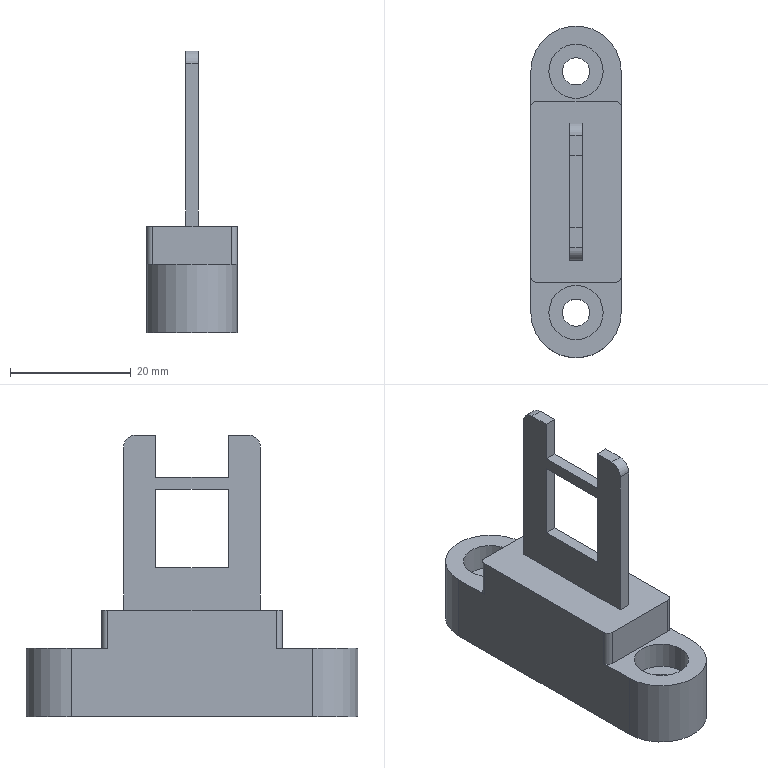Part | NX | 1 solid | 35 faces | box 15 x 55 x 46.7 mm | volume 11725 mm3 | plane 23 | cylinder 12 | commonest cylinder face diameters 2 x4 4 x2 4.5 x2 9 x2 15 x2
STEP:
#1=CARTESIAN_POINT('',(1.,10.65,46.7));
#2=VERTEX_POINT('',#1);
#3=CARTESIAN_POINT('',(1.,14.,46.7));
#4=VERTEX_POINT('',#3);
#5=CARTESIAN_POINT('',(1.,8.65,46.7));
#6=DIRECTION('',(0.,1.,0.));
#7=VECTOR('',#6,1000.);
#8=LINE('',#5,#7);
#9=EDGE_CURVE('',#2,#4,#8,.T.);
#10=ORIENTED_EDGE('',*,*,#9,.T.);
#11=CARTESIAN_POINT('',(-1.,14.,46.7));
#12=VERTEX_POINT('',#11);
#13=CARTESIAN_POINT('',(0.,14.,46.7));
#14=DIRECTION('',(-1.,0.,0.));
#15=VECTOR('',#14,1000.);
#16=LINE('',#13,#15);
#17=EDGE_CURVE('',#4,#12,#16,.T.);
#18=ORIENTED_EDGE('',*,*,#17,.T.);
#19=CARTESIAN_POINT('',(-1.,10.65,46.7));
#20=VERTEX_POINT('',#19);
#21=CARTESIAN_POINT('',(-1.,8.65,46.7));
#22=DIRECTION('',(0.,-1.,0.));
#23=VECTOR('',#22,1000.);
#24=LINE('',#21,#23);
#25=EDGE_CURVE('',#12,#20,#24,.T.);
#26=ORIENTED_EDGE('',*,*,#25,.T.);
#27=CARTESIAN_POINT('',(0.,10.65,46.7));
#28=DIRECTION('',(1.,0.,0.));
#29=VECTOR('',#28,1000.);
#30=LINE('',#27,#29);
#31=EDGE_CURVE('',#20,#2,#30,.T.);
#32=ORIENTED_EDGE('',*,*,#31,.T.);
#33=EDGE_LOOP('',(#10,#18,#26,#32));
#34=FACE_BOUND('',#33,.T.);
#35=CARTESIAN_POINT('',(0.,0.,46.7));
#36=DIRECTION('',(0.,0.,-1.));
#37=DIRECTION('',(-1.,0.,0.));
#38=AXIS2_PLACEMENT_3D('',#35,#36,#37);
#39=PLANE('',#38);
#40=ADVANCED_FACE('',(#34),#39,.F.);
#41=CARTESIAN_POINT('',(-7.5,34.,17.7));
#42=VERTEX_POINT('',#41);
#43=CARTESIAN_POINT('',(-7.5,6.,17.7));
#44=VERTEX_POINT('',#43);
#45=CARTESIAN_POINT('',(-7.5,0.,17.7));
#46=DIRECTION('',(0.,-1.,0.));
#47=VECTOR('',#46,1000.);
#48=LINE('',#45,#47);
#49=EDGE_CURVE('',#42,#44,#48,.T.);
#50=ORIENTED_EDGE('',*,*,#49,.T.);
#51=CARTESIAN_POINT('',(-6.5,5.,17.7));
#52=VERTEX_POINT('',#51);
#53=CARTESIAN_POINT('',(-6.5,6.,17.7));
#54=DIRECTION('',(0.,0.,1.));
#55=DIRECTION('',(1.,0.,0.));
#56=AXIS2_PLACEMENT_3D('',#53,#54,#55);
#57=CIRCLE('',#56,1.);
#58=EDGE_CURVE('',#44,#52,#57,.T.);
#59=ORIENTED_EDGE('',*,*,#58,.T.);
#60=CARTESIAN_POINT('',(6.5,5.,17.7));
#61=VERTEX_POINT('',#60);
#62=CARTESIAN_POINT('',(-7.5,5.,17.7));
#63=DIRECTION('',(-1.,0.,0.));
#64=VECTOR('',#63,1000.);
#65=LINE('',#62,#64);
#66=EDGE_CURVE('',#61,#52,#65,.T.);
#67=ORIENTED_EDGE('',*,*,#66,.F.);
#68=CARTESIAN_POINT('',(7.5,6.,17.7));
#69=VERTEX_POINT('',#68);
#70=CARTESIAN_POINT('',(6.5,6.,17.7));
#71=DIRECTION('',(0.,0.,1.));
#72=DIRECTION('',(1.,0.,0.));
#73=AXIS2_PLACEMENT_3D('',#70,#71,#72);
#74=CIRCLE('',#73,1.);
#75=EDGE_CURVE('',#61,#69,#74,.T.);
#76=ORIENTED_EDGE('',*,*,#75,.T.);
#77=CARTESIAN_POINT('',(7.5,34.,17.7));
#78=VERTEX_POINT('',#77);
#79=CARTESIAN_POINT('',(7.5,0.,17.7));
#80=DIRECTION('',(0.,1.,0.));
#81=VECTOR('',#80,1000.);
#82=LINE('',#79,#81);
#83=EDGE_CURVE('',#69,#78,#82,.T.);
#84=ORIENTED_EDGE('',*,*,#83,.T.);
#85=CARTESIAN_POINT('',(6.5,35.,17.7));
#86=VERTEX_POINT('',#85);
#87=CARTESIAN_POINT('',(6.5,34.,17.7));
#88=DIRECTION('',(0.,0.,1.));
#89=DIRECTION('',(1.,0.,0.));
#90=AXIS2_PLACEMENT_3D('',#87,#88,#89);
#91=CIRCLE('',#90,1.);
#92=EDGE_CURVE('',#78,#86,#91,.T.);
#93=ORIENTED_EDGE('',*,*,#92,.T.);
#94=CARTESIAN_POINT('',(-6.5,35.,17.7));
#95=VERTEX_POINT('',#94);
#96=CARTESIAN_POINT('',(7.5,35.,17.7));
#97=DIRECTION('',(1.,0.,0.));
#98=VECTOR('',#97,1000.);
#99=LINE('',#96,#98);
#100=EDGE_CURVE('',#95,#86,#99,.T.);
#101=ORIENTED_EDGE('',*,*,#100,.F.);
#102=CARTESIAN_POINT('',(-6.5,34.,17.7));
#103=DIRECTION('',(0.,0.,1.));
#104=DIRECTION('',(1.,0.,0.));
#105=AXIS2_PLACEMENT_3D('',#102,#103,#104);
#106=CIRCLE('',#105,1.);
#107=EDGE_CURVE('',#95,#42,#106,.T.);
#108=ORIENTED_EDGE('',*,*,#107,.T.);
#109=EDGE_LOOP('',(#50,#59,#67,#76,#84,#93,#101,#108));
#110=FACE_BOUND('',#109,.T.);
#111=CARTESIAN_POINT('',(1.,31.35,17.7));
#112=VERTEX_POINT('',#111);
#113=CARTESIAN_POINT('',(-1.,31.35,17.7));
#114=VERTEX_POINT('',#113);
#115=CARTESIAN_POINT('',(-1.,31.35,17.7));
#116=DIRECTION('',(-1.,0.,0.));
#117=VECTOR('',#116,1000.);
#118=LINE('',#115,#117);
#119=EDGE_CURVE('',#112,#114,#118,.T.);
#120=ORIENTED_EDGE('',*,*,#119,.F.);
#121=CARTESIAN_POINT('',(1.,8.65,17.7));
#122=VERTEX_POINT('',#121);
#123=CARTESIAN_POINT('',(1.,8.65,17.7));
#124=DIRECTION('',(0.,1.,0.));
#125=VECTOR('',#124,1000.);
#126=LINE('',#123,#125);
#127=EDGE_CURVE('',#122,#112,#126,.T.);
#128=ORIENTED_EDGE('',*,*,#127,.F.);
#129=CARTESIAN_POINT('',(-1.,8.65,17.7));
#130=VERTEX_POINT('',#129);
#131=CARTESIAN_POINT('',(-1.,8.65,17.7));
#132=DIRECTION('',(1.,0.,0.));
#133=VECTOR('',#132,1000.);
#134=LINE('',#131,#133);
#135=EDGE_CURVE('',#130,#122,#134,.T.);
#136=ORIENTED_EDGE('',*,*,#135,.F.);
#137=CARTESIAN_POINT('',(-1.,8.65,17.7));
#138=DIRECTION('',(0.,-1.,0.));
#139=VECTOR('',#138,1000.);
#140=LINE('',#137,#139);
#141=EDGE_CURVE('',#114,#130,#140,.T.);
#142=ORIENTED_EDGE('',*,*,#141,.F.);
#143=EDGE_LOOP('',(#120,#128,#136,#142));
#144=FACE_BOUND('',#143,.T.);
#145=CARTESIAN_POINT('',(0.,0.,17.7));
#146=DIRECTION('',(0.,0.,1.));
#147=DIRECTION('',(1.,0.,0.));
#148=AXIS2_PLACEMENT_3D('',#145,#146,#147);
#149=PLANE('',#148);
#150=ADVANCED_FACE('',(#110,#144),#149,.T.);
#151=CARTESIAN_POINT('',(-7.5,0.,11.4));
#152=VERTEX_POINT('',#151);
#153=CARTESIAN_POINT('',(7.5,0.,11.4));
#154=VERTEX_POINT('',#153);
#155=CARTESIAN_POINT('',(0.,0.,11.4));
#156=DIRECTION('',(0.,0.,1.));
#157=DIRECTION('',(1.,0.,0.));
#158=AXIS2_PLACEMENT_3D('',#155,#156,#157);
#159=CIRCLE('',#158,7.5);
#160=EDGE_CURVE('',#152,#154,#159,.T.);
#161=ORIENTED_EDGE('',*,*,#160,.F.);
#162=CARTESIAN_POINT('',(-7.5,0.,0.));
#163=VERTEX_POINT('',#162);
#164=CARTESIAN_POINT('',(-7.5,0.,17.7));
#165=DIRECTION('',(0.,0.,-1.));
#166=VECTOR('',#165,1000.);
#167=LINE('',#164,#166);
#168=EDGE_CURVE('',#152,#163,#167,.T.);
#169=ORIENTED_EDGE('',*,*,#168,.T.);
#170=CARTESIAN_POINT('',(7.5,0.,0.));
#171=VERTEX_POINT('',#170);
#172=CARTESIAN_POINT('',(0.,0.,0.));
#173=DIRECTION('',(0.,0.,1.));
#174=DIRECTION('',(1.,0.,0.));
#175=AXIS2_PLACEMENT_3D('',#172,#173,#174);
#176=CIRCLE('',#175,7.5);
#177=EDGE_CURVE('',#163,#171,#176,.T.);
#178=ORIENTED_EDGE('',*,*,#177,.T.);
#179=CARTESIAN_POINT('',(7.5,0.,17.7));
#180=DIRECTION('',(0.,0.,-1.));
#181=VECTOR('',#180,1000.);
#182=LINE('',#179,#181);
#183=EDGE_CURVE('',#154,#171,#182,.T.);
#184=ORIENTED_EDGE('',*,*,#183,.F.);
#185=EDGE_LOOP('',(#161,#169,#178,#184));
#186=FACE_BOUND('',#185,.T.);
#187=CARTESIAN_POINT('',(0.,0.,17.7));
#188=DIRECTION('',(0.,0.,-1.));
#189=DIRECTION('',(-1.,0.,0.));
#190=AXIS2_PLACEMENT_3D('',#187,#188,#189);
#191=CYLINDRICAL_SURFACE('',#190,7.5);
#192=ADVANCED_FACE('',(#186),#191,.T.);
#193=CARTESIAN_POINT('',(7.5,40.,11.4));
#194=VERTEX_POINT('',#193);
#195=CARTESIAN_POINT('',(-7.5,40.,11.4));
#196=VERTEX_POINT('',#195);
#197=CARTESIAN_POINT('',(0.,40.,11.4));
#198=DIRECTION('',(0.,0.,1.));
#199=DIRECTION('',(1.,0.,0.));
#200=AXIS2_PLACEMENT_3D('',#197,#198,#199);
#201=CIRCLE('',#200,7.5);
#202=EDGE_CURVE('',#194,#196,#201,.T.);
#203=ORIENTED_EDGE('',*,*,#202,.F.);
#204=CARTESIAN_POINT('',(7.5,40.,0.));
#205=VERTEX_POINT('',#204);
#206=CARTESIAN_POINT('',(7.5,40.,17.7));
#207=DIRECTION('',(0.,0.,-1.));
#208=VECTOR('',#207,1000.);
#209=LINE('',#206,#208);
#210=EDGE_CURVE('',#194,#205,#209,.T.);
#211=ORIENTED_EDGE('',*,*,#210,.T.);
#212=CARTESIAN_POINT('',(-7.5,40.,0.));
#213=VERTEX_POINT('',#212);
#214=CARTESIAN_POINT('',(0.,40.,0.));
#215=DIRECTION('',(0.,0.,1.));
#216=DIRECTION('',(1.,0.,0.));
#217=AXIS2_PLACEMENT_3D('',#214,#215,#216);
#218=CIRCLE('',#217,7.5);
#219=EDGE_CURVE('',#205,#213,#218,.T.);
#220=ORIENTED_EDGE('',*,*,#219,.T.);
#221=CARTESIAN_POINT('',(-7.5,40.,17.7));
#222=DIRECTION('',(0.,0.,-1.));
#223=VECTOR('',#222,1000.);
#224=LINE('',#221,#223);
#225=EDGE_CURVE('',#196,#213,#224,.T.);
#226=ORIENTED_EDGE('',*,*,#225,.F.);
#227=EDGE_LOOP('',(#203,#211,#220,#226));
#228=FACE_BOUND('',#227,.T.);
#229=CARTESIAN_POINT('',(0.,40.,17.7));
#230=DIRECTION('',(0.,0.,-1.));
#231=DIRECTION('',(-1.,0.,0.));
#232=AXIS2_PLACEMENT_3D('',#229,#230,#231);
#233=CYLINDRICAL_SURFACE('',#232,7.5);
#234=ADVANCED_FACE('',(#228),#233,.T.);
#235=ORIENTED_EDGE('',*,*,#83,.F.);
#236=CARTESIAN_POINT('',(7.5,6.,11.4));
#237=VERTEX_POINT('',#236);
#238=CARTESIAN_POINT('',(7.5,6.,17.7));
#239=DIRECTION('',(0.,0.,1.));
#240=VECTOR('',#239,1000.);
#241=LINE('',#238,#240);
#242=EDGE_CURVE('',#69,#237,#241,.F.);
#243=ORIENTED_EDGE('',*,*,#242,.T.);
#244=CARTESIAN_POINT('',(7.5,5.,11.4));
#245=DIRECTION('',(0.,1.,0.));
#246=VECTOR('',#245,1000.);
#247=LINE('',#244,#246);
#248=EDGE_CURVE('',#154,#237,#247,.T.);
#249=ORIENTED_EDGE('',*,*,#248,.F.);
#250=ORIENTED_EDGE('',*,*,#183,.T.);
#251=CARTESIAN_POINT('',(7.5,0.,0.));
#252=DIRECTION('',(0.,1.,0.));
#253=VECTOR('',#252,1000.);
#254=LINE('',#251,#253);
#255=EDGE_CURVE('',#171,#205,#254,.T.);
#256=ORIENTED_EDGE('',*,*,#255,.T.);
#257=ORIENTED_EDGE('',*,*,#210,.F.);
#258=CARTESIAN_POINT('',(7.5,34.,11.4));
#259=VERTEX_POINT('',#258);
#260=CARTESIAN_POINT('',(7.5,35.,11.4));
#261=DIRECTION('',(0.,1.,0.));
#262=VECTOR('',#261,1000.);
#263=LINE('',#260,#262);
#264=EDGE_CURVE('',#259,#194,#263,.T.);
#265=ORIENTED_EDGE('',*,*,#264,.F.);
#266=CARTESIAN_POINT('',(7.5,34.,17.7));
#267=DIRECTION('',(0.,0.,1.));
#268=VECTOR('',#267,1000.);
#269=LINE('',#266,#268);
#270=EDGE_CURVE('',#259,#78,#269,.T.);
#271=ORIENTED_EDGE('',*,*,#270,.T.);
#272=EDGE_LOOP('',(#235,#243,#249,#250,#256,#257,#265,#271));
#273=FACE_BOUND('',#272,.T.);
#274=CARTESIAN_POINT('',(7.5,0.,17.7));
#275=DIRECTION('',(-1.,0.,0.));
#276=DIRECTION('',(0.,0.,1.));
#277=AXIS2_PLACEMENT_3D('',#274,#275,#276);
#278=PLANE('',#277);
#279=ADVANCED_FACE('',(#273),#278,.F.);
#280=CARTESIAN_POINT('',(-7.5,6.,11.4));
#281=VERTEX_POINT('',#280);
#282=CARTESIAN_POINT('',(-7.5,5.,11.4));
#283=DIRECTION('',(0.,-1.,0.));
#284=VECTOR('',#283,1000.);
#285=LINE('',#282,#284);
#286=EDGE_CURVE('',#281,#152,#285,.T.);
#287=ORIENTED_EDGE('',*,*,#286,.F.);
#288=CARTESIAN_POINT('',(-7.5,6.,17.7));
#289=DIRECTION('',(0.,0.,1.));
#290=VECTOR('',#289,1000.);
#291=LINE('',#288,#290);
#292=EDGE_CURVE('',#281,#44,#291,.T.);
#293=ORIENTED_EDGE('',*,*,#292,.T.);
#294=ORIENTED_EDGE('',*,*,#49,.F.);
#295=CARTESIAN_POINT('',(-7.5,34.,11.4));
#296=VERTEX_POINT('',#295);
#297=CARTESIAN_POINT('',(-7.5,34.,17.7));
#298=DIRECTION('',(0.,0.,1.));
#299=VECTOR('',#298,1000.);
#300=LINE('',#297,#299);
#301=EDGE_CURVE('',#42,#296,#300,.F.);
#302=ORIENTED_EDGE('',*,*,#301,.T.);
#303=CARTESIAN_POINT('',(-7.5,35.,11.4));
#304=DIRECTION('',(0.,-1.,0.));
#305=VECTOR('',#304,1000.);
#306=LINE('',#303,#305);
#307=EDGE_CURVE('',#196,#296,#306,.T.);
#308=ORIENTED_EDGE('',*,*,#307,.F.);
#309=ORIENTED_EDGE('',*,*,#225,.T.);
#310=CARTESIAN_POINT('',(-7.5,0.,0.));
#311=DIRECTION('',(0.,-1.,0.));
#312=VECTOR('',#311,1000.);
#313=LINE('',#310,#312);
#314=EDGE_CURVE('',#213,#163,#313,.T.);
#315=ORIENTED_EDGE('',*,*,#314,.T.);
#316=ORIENTED_EDGE('',*,*,#168,.F.);
#317=EDGE_LOOP('',(#287,#293,#294,#302,#308,#309,#315,#316));
#318=FACE_BOUND('',#317,.T.);
#319=CARTESIAN_POINT('',(-7.5,0.,17.7));
#320=DIRECTION('',(1.,0.,0.));
#321=DIRECTION('',(0.,0.,-1.));
#322=AXIS2_PLACEMENT_3D('',#319,#320,#321);
#323=PLANE('',#322);
#324=ADVANCED_FACE('',(#318),#323,.F.);
#325=CARTESIAN_POINT('',(2.25,0.,0.));
#326=VERTEX_POINT('',#325);
#327=CARTESIAN_POINT('',(0.,0.,0.));
#328=DIRECTION('',(0.,0.,1.));
#329=DIRECTION('',(1.,0.,0.));
#330=AXIS2_PLACEMENT_3D('',#327,#328,#329);
#331=CIRCLE('',#330,2.25);
#332=EDGE_CURVE('',#326,#326,#331,.T.);
#333=ORIENTED_EDGE('',*,*,#332,.T.);
#334=EDGE_LOOP('',(#333));
#335=FACE_BOUND('',#334,.T.);
#336=CARTESIAN_POINT('',(2.25,40.,0.));
#337=VERTEX_POINT('',#336);
#338=CARTESIAN_POINT('',(0.,40.,0.));
#339=DIRECTION('',(0.,0.,1.));
#340=DIRECTION('',(1.,0.,0.));
#341=AXIS2_PLACEMENT_3D('',#338,#339,#340);
#342=CIRCLE('',#341,2.25);
#343=EDGE_CURVE('',#337,#337,#342,.T.);
#344=ORIENTED_EDGE('',*,*,#343,.T.);
#345=EDGE_LOOP('',(#344));
#346=FACE_BOUND('',#345,.T.);
#347=ORIENTED_EDGE('',*,*,#177,.F.);
#348=ORIENTED_EDGE('',*,*,#314,.F.);
#349=ORIENTED_EDGE('',*,*,#219,.F.);
#350=ORIENTED_EDGE('',*,*,#255,.F.);
#351=EDGE_LOOP('',(#347,#348,#349,#350));
#352=FACE_BOUND('',#351,.T.);
#353=CARTESIAN_POINT('',(0.,0.,0.));
#354=DIRECTION('',(0.,0.,1.));
#355=DIRECTION('',(1.,0.,0.));
#356=AXIS2_PLACEMENT_3D('',#353,#354,#355);
#357=PLANE('',#356);
#358=ADVANCED_FACE('',(#335,#346,#352),#357,.F.);
#359=CARTESIAN_POINT('',(4.5,40.,11.4));
#360=VERTEX_POINT('',#359);
#361=CARTESIAN_POINT('',(0.,40.,11.4));
#362=DIRECTION('',(0.,0.,1.));
#363=DIRECTION('',(1.,0.,0.));
#364=AXIS2_PLACEMENT_3D('',#361,#362,#363);
#365=CIRCLE('',#364,4.5);
#366=EDGE_CURVE('',#360,#360,#365,.T.);
#367=ORIENTED_EDGE('',*,*,#366,.F.);
#368=EDGE_LOOP('',(#367));
#369=FACE_BOUND('',#368,.T.);
#370=ORIENTED_EDGE('',*,*,#202,.T.);
#371=ORIENTED_EDGE('',*,*,#307,.T.);
#372=CARTESIAN_POINT('',(-6.5,35.,11.4));
#373=VERTEX_POINT('',#372);
#374=CARTESIAN_POINT('',(-6.5,34.,11.4));
#375=DIRECTION('',(0.,0.,1.));
#376=DIRECTION('',(1.,0.,0.));
#377=AXIS2_PLACEMENT_3D('',#374,#375,#376);
#378=CIRCLE('',#377,1.);
#379=EDGE_CURVE('',#296,#373,#378,.F.);
#380=ORIENTED_EDGE('',*,*,#379,.T.);
#381=CARTESIAN_POINT('',(6.5,35.,11.4));
#382=VERTEX_POINT('',#381);
#383=CARTESIAN_POINT('',(7.5,35.,11.4));
#384=DIRECTION('',(1.,0.,0.));
#385=VECTOR('',#384,1000.);
#386=LINE('',#383,#385);
#387=EDGE_CURVE('',#373,#382,#386,.T.);
#388=ORIENTED_EDGE('',*,*,#387,.T.);
#389=CARTESIAN_POINT('',(6.5,34.,11.4));
#390=DIRECTION('',(0.,0.,1.));
#391=DIRECTION('',(1.,0.,0.));
#392=AXIS2_PLACEMENT_3D('',#389,#390,#391);
#393=CIRCLE('',#392,1.);
#394=EDGE_CURVE('',#382,#259,#393,.F.);
#395=ORIENTED_EDGE('',*,*,#394,.T.);
#396=ORIENTED_EDGE('',*,*,#264,.T.);
#397=EDGE_LOOP('',(#370,#371,#380,#388,#395,#396));
#398=FACE_BOUND('',#397,.T.);
#399=CARTESIAN_POINT('',(0.,0.,11.4));
#400=DIRECTION('',(0.,0.,1.));
#401=DIRECTION('',(1.,0.,0.));
#402=AXIS2_PLACEMENT_3D('',#399,#400,#401);
#403=PLANE('',#402);
#404=ADVANCED_FACE('',(#369,#398),#403,.T.);
#405=ORIENTED_EDGE('',*,*,#100,.T.);
#406=CARTESIAN_POINT('',(6.5,35.,11.4));
#407=DIRECTION('',(0.,0.,1.));
#408=VECTOR('',#407,1000.);
#409=LINE('',#406,#408);
#410=EDGE_CURVE('',#86,#382,#409,.F.);
#411=ORIENTED_EDGE('',*,*,#410,.T.);
#412=ORIENTED_EDGE('',*,*,#387,.F.);
#413=CARTESIAN_POINT('',(-6.5,35.,11.4));
#414=DIRECTION('',(0.,0.,1.));
#415=VECTOR('',#414,1000.);
#416=LINE('',#413,#415);
#417=EDGE_CURVE('',#373,#95,#416,.T.);
#418=ORIENTED_EDGE('',*,*,#417,.T.);
#419=EDGE_LOOP('',(#405,#411,#412,#418));
#420=FACE_BOUND('',#419,.T.);
#421=CARTESIAN_POINT('',(7.5,35.,11.4));
#422=DIRECTION('',(0.,-1.,0.));
#423=DIRECTION('',(0.,0.,-1.));
#424=AXIS2_PLACEMENT_3D('',#421,#422,#423);
#425=PLANE('',#424);
#426=ADVANCED_FACE('',(#420),#425,.F.);
#427=CARTESIAN_POINT('',(4.5,0.,11.4));
#428=VERTEX_POINT('',#427);
#429=CARTESIAN_POINT('',(0.,0.,11.4));
#430=DIRECTION('',(0.,0.,1.));
#431=DIRECTION('',(1.,0.,0.));
#432=AXIS2_PLACEMENT_3D('',#429,#430,#431);
#433=CIRCLE('',#432,4.5);
#434=EDGE_CURVE('',#428,#428,#433,.T.);
#435=ORIENTED_EDGE('',*,*,#434,.F.);
#436=EDGE_LOOP('',(#435));
#437=FACE_BOUND('',#436,.T.);
#438=ORIENTED_EDGE('',*,*,#160,.T.);
#439=ORIENTED_EDGE('',*,*,#248,.T.);
#440=CARTESIAN_POINT('',(6.5,5.,11.4));
#441=VERTEX_POINT('',#440);
#442=CARTESIAN_POINT('',(6.5,6.,11.4));
#443=DIRECTION('',(0.,0.,1.));
#444=DIRECTION('',(1.,0.,0.));
#445=AXIS2_PLACEMENT_3D('',#442,#443,#444);
#446=CIRCLE('',#445,1.);
#447=EDGE_CURVE('',#237,#441,#446,.F.);
#448=ORIENTED_EDGE('',*,*,#447,.T.);
#449=CARTESIAN_POINT('',(-6.5,5.,11.4));
#450=VERTEX_POINT('',#449);
#451=CARTESIAN_POINT('',(-7.5,5.,11.4));
#452=DIRECTION('',(-1.,0.,0.));
#453=VECTOR('',#452,1000.);
#454=LINE('',#451,#453);
#455=EDGE_CURVE('',#441,#450,#454,.T.);
#456=ORIENTED_EDGE('',*,*,#455,.T.);
#457=CARTESIAN_POINT('',(-6.5,6.,11.4));
#458=DIRECTION('',(0.,0.,1.));
#459=DIRECTION('',(1.,0.,0.));
#460=AXIS2_PLACEMENT_3D('',#457,#458,#459);
#461=CIRCLE('',#460,1.);
#462=EDGE_CURVE('',#450,#281,#461,.F.);
#463=ORIENTED_EDGE('',*,*,#462,.T.);
#464=ORIENTED_EDGE('',*,*,#286,.T.);
#465=EDGE_LOOP('',(#438,#439,#448,#456,#463,#464));
#466=FACE_BOUND('',#465,.T.);
#467=CARTESIAN_POINT('',(0.,0.,11.4));
#468=DIRECTION('',(0.,0.,1.));
#469=DIRECTION('',(1.,0.,0.));
#470=AXIS2_PLACEMENT_3D('',#467,#468,#469);
#471=PLANE('',#470);
#472=ADVANCED_FACE('',(#437,#466),#471,.T.);
#473=ORIENTED_EDGE('',*,*,#66,.T.);
#474=CARTESIAN_POINT('',(-6.5,5.,11.4));
#475=DIRECTION('',(0.,0.,1.));
#476=VECTOR('',#475,1000.);
#477=LINE('',#474,#476);
#478=EDGE_CURVE('',#52,#450,#477,.F.);
#479=ORIENTED_EDGE('',*,*,#478,.T.);
#480=ORIENTED_EDGE('',*,*,#455,.F.);
#481=CARTESIAN_POINT('',(6.5,5.,11.4));
#482=DIRECTION('',(0.,0.,1.));
#483=VECTOR('',#482,1000.);
#484=LINE('',#481,#483);
#485=EDGE_CURVE('',#441,#61,#484,.T.);
#486=ORIENTED_EDGE('',*,*,#485,.T.);
#487=EDGE_LOOP('',(#473,#479,#480,#486));
#488=FACE_BOUND('',#487,.T.);
#489=CARTESIAN_POINT('',(-7.5,5.,11.4));
#490=DIRECTION('',(0.,1.,0.));
#491=DIRECTION('',(-1.,0.,0.));
#492=AXIS2_PLACEMENT_3D('',#489,#490,#491);
#493=PLANE('',#492);
#494=ADVANCED_FACE('',(#488),#493,.F.);
#495=ORIENTED_EDGE('',*,*,#462,.F.);
#496=ORIENTED_EDGE('',*,*,#478,.F.);
#497=ORIENTED_EDGE('',*,*,#58,.F.);
#498=ORIENTED_EDGE('',*,*,#292,.F.);
#499=EDGE_LOOP('',(#495,#496,#497,#498));
#500=FACE_BOUND('',#499,.T.);
#501=CARTESIAN_POINT('',(-6.5,6.,17.7));
#502=DIRECTION('',(0.,0.,1.));
#503=DIRECTION('',(1.,0.,0.));
#504=AXIS2_PLACEMENT_3D('',#501,#502,#503);
#505=CYLINDRICAL_SURFACE('',#504,1.);
#506=ADVANCED_FACE('',(#500),#505,.T.);
#507=ORIENTED_EDGE('',*,*,#447,.F.);
#508=ORIENTED_EDGE('',*,*,#242,.F.);
#509=ORIENTED_EDGE('',*,*,#75,.F.);
#510=ORIENTED_EDGE('',*,*,#485,.F.);
#511=EDGE_LOOP('',(#507,#508,#509,#510));
#512=FACE_BOUND('',#511,.T.);
#513=CARTESIAN_POINT('',(6.5,6.,11.4));
#514=DIRECTION('',(0.,0.,1.));
#515=DIRECTION('',(1.,0.,0.));
#516=AXIS2_PLACEMENT_3D('',#513,#514,#515);
#517=CYLINDRICAL_SURFACE('',#516,1.);
#518=ADVANCED_FACE('',(#512),#517,.T.);
#519=ORIENTED_EDGE('',*,*,#394,.F.);
#520=ORIENTED_EDGE('',*,*,#410,.F.);
#521=ORIENTED_EDGE('',*,*,#92,.F.);
#522=ORIENTED_EDGE('',*,*,#270,.F.);
#523=EDGE_LOOP('',(#519,#520,#521,#522));
#524=FACE_BOUND('',#523,.T.);
#525=CARTESIAN_POINT('',(6.5,34.,17.7));
#526=DIRECTION('',(0.,0.,1.));
#527=DIRECTION('',(1.,0.,0.));
#528=AXIS2_PLACEMENT_3D('',#525,#526,#527);
#529=CYLINDRICAL_SURFACE('',#528,1.);
#530=ADVANCED_FACE('',(#524),#529,.T.);
#531=ORIENTED_EDGE('',*,*,#379,.F.);
#532=ORIENTED_EDGE('',*,*,#301,.F.);
#533=ORIENTED_EDGE('',*,*,#107,.F.);
#534=ORIENTED_EDGE('',*,*,#417,.F.);
#535=EDGE_LOOP('',(#531,#532,#533,#534));
#536=FACE_BOUND('',#535,.T.);
#537=CARTESIAN_POINT('',(-6.5,34.,11.4));
#538=DIRECTION('',(0.,0.,1.));
#539=DIRECTION('',(1.,0.,0.));
#540=AXIS2_PLACEMENT_3D('',#537,#538,#539);
#541=CYLINDRICAL_SURFACE('',#540,1.);
#542=ADVANCED_FACE('',(#536),#541,.T.);
#543=CARTESIAN_POINT('',(1.,14.,24.7));
#544=VERTEX_POINT('',#543);
#545=CARTESIAN_POINT('',(1.,14.,37.7));
#546=VERTEX_POINT('',#545);
#547=CARTESIAN_POINT('',(1.,14.,46.7));
#548=DIRECTION('',(0.,0.,1.));
#549=VECTOR('',#548,1000.);
#550=LINE('',#547,#549);
#551=EDGE_CURVE('',#544,#546,#550,.T.);
#552=ORIENTED_EDGE('',*,*,#551,.T.);
#553=CARTESIAN_POINT('',(1.,26.,37.7));
#554=VERTEX_POINT('',#553);
#555=CARTESIAN_POINT('',(1.,8.65,37.7));
#556=DIRECTION('',(0.,1.,0.));
#557=VECTOR('',#556,1000.);
#558=LINE('',#555,#557);
#559=EDGE_CURVE('',#546,#554,#558,.T.);
#560=ORIENTED_EDGE('',*,*,#559,.T.);
#561=CARTESIAN_POINT('',(1.,26.,24.7));
#562=VERTEX_POINT('',#561);
#563=CARTESIAN_POINT('',(1.,26.,46.7));
#564=DIRECTION('',(0.,0.,-1.));
#565=VECTOR('',#564,1000.);
#566=LINE('',#563,#565);
#567=EDGE_CURVE('',#554,#562,#566,.T.);
#568=ORIENTED_EDGE('',*,*,#567,.T.);
#569=CARTESIAN_POINT('',(1.,8.65,24.7));
#570=DIRECTION('',(0.,-1.,0.));
#571=VECTOR('',#570,1000.);
#572=LINE('',#569,#571);
#573=EDGE_CURVE('',#562,#544,#572,.T.);
#574=ORIENTED_EDGE('',*,*,#573,.T.);
#575=EDGE_LOOP('',(#552,#560,#568,#574));
#576=FACE_BOUND('',#575,.T.);
#577=CARTESIAN_POINT('',(1.,26.,39.7));
#578=VERTEX_POINT('',#577);
#579=CARTESIAN_POINT('',(1.,14.,39.7));
#580=VERTEX_POINT('',#579);
#581=CARTESIAN_POINT('',(1.,8.65,39.7));
#582=DIRECTION('',(0.,-1.,0.));
#583=VECTOR('',#582,1000.);
#584=LINE('',#581,#583);
#585=EDGE_CURVE('',#578,#580,#584,.T.);
#586=ORIENTED_EDGE('',*,*,#585,.T.);
#587=CARTESIAN_POINT('',(1.,14.,46.7));
#588=DIRECTION('',(0.,0.,1.));
#589=VECTOR('',#588,1000.);
#590=LINE('',#587,#589);
#591=EDGE_CURVE('',#580,#4,#590,.T.);
#592=ORIENTED_EDGE('',*,*,#591,.T.);
#593=ORIENTED_EDGE('',*,*,#9,.F.);
#594=CARTESIAN_POINT('',(1.,8.65,44.7));
#595=VERTEX_POINT('',#594);
#596=CARTESIAN_POINT('',(1.,10.65,44.7));
#597=DIRECTION('',(-1.,0.,0.));
#598=DIRECTION('',(0.,0.,1.));
#599=AXIS2_PLACEMENT_3D('',#596,#597,#598);
#600=CIRCLE('',#599,2.);
#601=EDGE_CURVE('',#2,#595,#600,.F.);
#602=ORIENTED_EDGE('',*,*,#601,.T.);
#603=CARTESIAN_POINT('',(1.,8.65,46.7));
#604=DIRECTION('',(0.,0.,-1.));
#605=VECTOR('',#604,1000.);
#606=LINE('',#603,#605);
#607=EDGE_CURVE('',#595,#122,#606,.T.);
#608=ORIENTED_EDGE('',*,*,#607,.T.);
#609=ORIENTED_EDGE('',*,*,#127,.T.);
#610=CARTESIAN_POINT('',(1.,31.35,44.7));
#611=VERTEX_POINT('',#610);
#612=CARTESIAN_POINT('',(1.,31.35,46.7));
#613=DIRECTION('',(0.,0.,-1.));
#614=VECTOR('',#613,1000.);
#615=LINE('',#612,#614);
#616=EDGE_CURVE('',#611,#112,#615,.T.);
#617=ORIENTED_EDGE('',*,*,#616,.F.);
#618=CARTESIAN_POINT('',(1.,29.35,46.7));
#619=VERTEX_POINT('',#618);
#620=CARTESIAN_POINT('',(1.,29.35,44.7));
#621=DIRECTION('',(-1.,0.,0.));
#622=DIRECTION('',(0.,0.,1.));
#623=AXIS2_PLACEMENT_3D('',#620,#621,#622);
#624=CIRCLE('',#623,2.);
#625=EDGE_CURVE('',#611,#619,#624,.F.);
#626=ORIENTED_EDGE('',*,*,#625,.T.);
#627=CARTESIAN_POINT('',(1.,26.,46.7));
#628=VERTEX_POINT('',#627);
#629=CARTESIAN_POINT('',(1.,8.65,46.7));
#630=DIRECTION('',(0.,1.,0.));
#631=VECTOR('',#630,1000.);
#632=LINE('',#629,#631);
#633=EDGE_CURVE('',#628,#619,#632,.T.);
#634=ORIENTED_EDGE('',*,*,#633,.F.);
#635=CARTESIAN_POINT('',(1.,26.,46.7));
#636=DIRECTION('',(0.,0.,-1.));
#637=VECTOR('',#636,1000.);
#638=LINE('',#635,#637);
#639=EDGE_CURVE('',#628,#578,#638,.T.);
#640=ORIENTED_EDGE('',*,*,#639,.T.);
#641=EDGE_LOOP('',(#586,#592,#593,#602,#608,#609,#617,#626,#634,#640));
#642=FACE_BOUND('',#641,.T.);
#643=CARTESIAN_POINT('',(1.,8.65,46.7));
#644=DIRECTION('',(-1.,0.,0.));
#645=DIRECTION('',(0.,0.,1.));
#646=AXIS2_PLACEMENT_3D('',#643,#644,#645);
#647=PLANE('',#646);
#648=ADVANCED_FACE('',(#576,#642),#647,.F.);
#649=CARTESIAN_POINT('',(-1.,31.35,44.7));
#650=VERTEX_POINT('',#649);
#651=CARTESIAN_POINT('',(-1.,31.35,46.7));
#652=DIRECTION('',(0.,0.,-1.));
#653=VECTOR('',#652,1000.);
#654=LINE('',#651,#653);
#655=EDGE_CURVE('',#650,#114,#654,.T.);
#656=ORIENTED_EDGE('',*,*,#655,.F.);
#657=CARTESIAN_POINT('',(-1.,31.35,44.7));
#658=DIRECTION('',(-1.,0.,0.));
#659=VECTOR('',#658,1000.);
#660=LINE('',#657,#659);
#661=EDGE_CURVE('',#650,#611,#660,.F.);
#662=ORIENTED_EDGE('',*,*,#661,.T.);
#663=ORIENTED_EDGE('',*,*,#616,.T.);
#664=ORIENTED_EDGE('',*,*,#119,.T.);
#665=EDGE_LOOP('',(#656,#662,#663,#664));
#666=FACE_BOUND('',#665,.T.);
#667=CARTESIAN_POINT('',(-1.,31.35,46.7));
#668=DIRECTION('',(0.,-1.,0.));
#669=DIRECTION('',(0.,0.,-1.));
#670=AXIS2_PLACEMENT_3D('',#667,#668,#669);
#671=PLANE('',#670);
#672=ADVANCED_FACE('',(#666),#671,.F.);
#673=CARTESIAN_POINT('',(-1.,26.,37.7));
#674=VERTEX_POINT('',#673);
#675=CARTESIAN_POINT('',(-1.,26.,24.7));
#676=VERTEX_POINT('',#675);
#677=CARTESIAN_POINT('',(-1.,26.,24.7));
#678=DIRECTION('',(0.,0.,-1.));
#679=VECTOR('',#678,1000.);
#680=LINE('',#677,#679);
#681=EDGE_CURVE('',#674,#676,#680,.T.);
#682=ORIENTED_EDGE('',*,*,#681,.F.);
#683=CARTESIAN_POINT('',(-1.,14.,37.7));
#684=VERTEX_POINT('',#683);
#685=CARTESIAN_POINT('',(-1.,14.,37.7));
#686=DIRECTION('',(0.,1.,0.));
#687=VECTOR('',#686,1000.);
#688=LINE('',#685,#687);
#689=EDGE_CURVE('',#684,#674,#688,.T.);
#690=ORIENTED_EDGE('',*,*,#689,.F.);
#691=CARTESIAN_POINT('',(-1.,14.,24.7));
#692=VERTEX_POINT('',#691);
#693=CARTESIAN_POINT('',(-1.,14.,24.7));
#694=DIRECTION('',(0.,0.,1.));
#695=VECTOR('',#694,1000.);
#696=LINE('',#693,#695);
#697=EDGE_CURVE('',#692,#684,#696,.T.);
#698=ORIENTED_EDGE('',*,*,#697,.F.);
#699=CARTESIAN_POINT('',(-1.,14.,24.7));
#700=DIRECTION('',(0.,-1.,0.));
#701=VECTOR('',#700,1000.);
#702=LINE('',#699,#701);
#703=EDGE_CURVE('',#676,#692,#702,.T.);
#704=ORIENTED_EDGE('',*,*,#703,.F.);
#705=EDGE_LOOP('',(#682,#690,#698,#704));
#706=FACE_BOUND('',#705,.T.);
#707=ORIENTED_EDGE('',*,*,#25,.F.);
#708=CARTESIAN_POINT('',(-1.,14.,39.7));
#709=VERTEX_POINT('',#708);
#710=CARTESIAN_POINT('',(-1.,14.,39.7));
#711=DIRECTION('',(0.,0.,1.));
#712=VECTOR('',#711,1000.);
#713=LINE('',#710,#712);
#714=EDGE_CURVE('',#709,#12,#713,.T.);
#715=ORIENTED_EDGE('',*,*,#714,.F.);
#716=CARTESIAN_POINT('',(-1.,26.,39.7));
#717=VERTEX_POINT('',#716);
#718=CARTESIAN_POINT('',(-1.,14.,39.7));
#719=DIRECTION('',(0.,-1.,0.));
#720=VECTOR('',#719,1000.);
#721=LINE('',#718,#720);
#722=EDGE_CURVE('',#717,#709,#721,.T.);
#723=ORIENTED_EDGE('',*,*,#722,.F.);
#724=CARTESIAN_POINT('',(-1.,26.,46.7));
#725=VERTEX_POINT('',#724);
#726=CARTESIAN_POINT('',(-1.,26.,39.7));
#727=DIRECTION('',(0.,0.,-1.));
#728=VECTOR('',#727,1000.);
#729=LINE('',#726,#728);
#730=EDGE_CURVE('',#725,#717,#729,.T.);
#731=ORIENTED_EDGE('',*,*,#730,.F.);
#732=CARTESIAN_POINT('',(-1.,29.35,46.7));
#733=VERTEX_POINT('',#732);
#734=CARTESIAN_POINT('',(-1.,8.65,46.7));
#735=DIRECTION('',(0.,-1.,0.));
#736=VECTOR('',#735,1000.);
#737=LINE('',#734,#736);
#738=EDGE_CURVE('',#733,#725,#737,.T.);
#739=ORIENTED_EDGE('',*,*,#738,.F.);
#740=CARTESIAN_POINT('',(-1.,29.35,44.7));
#741=DIRECTION('',(1.,0.,0.));
#742=DIRECTION('',(0.,0.,-1.));
#743=AXIS2_PLACEMENT_3D('',#740,#741,#742);
#744=CIRCLE('',#743,2.);
#745=EDGE_CURVE('',#733,#650,#744,.F.);
#746=ORIENTED_EDGE('',*,*,#745,.T.);
#747=ORIENTED_EDGE('',*,*,#655,.T.);
#748=ORIENTED_EDGE('',*,*,#141,.T.);
#749=CARTESIAN_POINT('',(-1.,8.65,44.7));
#750=VERTEX_POINT('',#749);
#751=CARTESIAN_POINT('',(-1.,8.65,46.7));
#752=DIRECTION('',(0.,0.,-1.));
#753=VECTOR('',#752,1000.);
#754=LINE('',#751,#753);
#755=EDGE_CURVE('',#750,#130,#754,.T.);
#756=ORIENTED_EDGE('',*,*,#755,.F.);
#757=CARTESIAN_POINT('',(-1.,10.65,44.7));
#758=DIRECTION('',(1.,0.,0.));
#759=DIRECTION('',(0.,0.,-1.));
#760=AXIS2_PLACEMENT_3D('',#757,#758,#759);
#761=CIRCLE('',#760,2.);
#762=EDGE_CURVE('',#750,#20,#761,.F.);
#763=ORIENTED_EDGE('',*,*,#762,.T.);
#764=EDGE_LOOP('',(#707,#715,#723,#731,#739,#746,#747,#748,#756,#763));
#765=FACE_BOUND('',#764,.T.);
#766=CARTESIAN_POINT('',(-1.,8.65,46.7));
#767=DIRECTION('',(1.,0.,0.));
#768=DIRECTION('',(0.,0.,-1.));
#769=AXIS2_PLACEMENT_3D('',#766,#767,#768);
#770=PLANE('',#769);
#771=ADVANCED_FACE('',(#706,#765),#770,.F.);
#772=ORIENTED_EDGE('',*,*,#607,.F.);
#773=CARTESIAN_POINT('',(-1.,8.65,44.7));
#774=DIRECTION('',(1.,0.,0.));
#775=VECTOR('',#774,1000.);
#776=LINE('',#773,#775);
#777=EDGE_CURVE('',#595,#750,#776,.F.);
#778=ORIENTED_EDGE('',*,*,#777,.T.);
#779=ORIENTED_EDGE('',*,*,#755,.T.);
#780=ORIENTED_EDGE('',*,*,#135,.T.);
#781=EDGE_LOOP('',(#772,#778,#779,#780));
#782=FACE_BOUND('',#781,.T.);
#783=CARTESIAN_POINT('',(-1.,8.65,46.7));
#784=DIRECTION('',(0.,1.,0.));
#785=DIRECTION('',(0.,0.,1.));
#786=AXIS2_PLACEMENT_3D('',#783,#784,#785);
#787=PLANE('',#786);
#788=ADVANCED_FACE('',(#782),#787,.F.);
#789=ORIENTED_EDGE('',*,*,#738,.T.);
#790=CARTESIAN_POINT('',(0.,26.,46.7));
#791=DIRECTION('',(1.,0.,0.));
#792=VECTOR('',#791,1000.);
#793=LINE('',#790,#792);
#794=EDGE_CURVE('',#725,#628,#793,.T.);
#795=ORIENTED_EDGE('',*,*,#794,.T.);
#796=ORIENTED_EDGE('',*,*,#633,.T.);
#797=CARTESIAN_POINT('',(0.,29.35,46.7));
#798=DIRECTION('',(-1.,0.,0.));
#799=VECTOR('',#798,1000.);
#800=LINE('',#797,#799);
#801=EDGE_CURVE('',#619,#733,#800,.T.);
#802=ORIENTED_EDGE('',*,*,#801,.T.);
#803=EDGE_LOOP('',(#789,#795,#796,#802));
#804=FACE_BOUND('',#803,.T.);
#805=CARTESIAN_POINT('',(0.,0.,46.7));
#806=DIRECTION('',(0.,0.,-1.));
#807=DIRECTION('',(-1.,0.,0.));
#808=AXIS2_PLACEMENT_3D('',#805,#806,#807);
#809=PLANE('',#808);
#810=ADVANCED_FACE('',(#804),#809,.F.);
#811=ORIENTED_EDGE('',*,*,#625,.F.);
#812=ORIENTED_EDGE('',*,*,#661,.F.);
#813=ORIENTED_EDGE('',*,*,#745,.F.);
#814=ORIENTED_EDGE('',*,*,#801,.F.);
#815=EDGE_LOOP('',(#811,#812,#813,#814));
#816=FACE_BOUND('',#815,.T.);
#817=CARTESIAN_POINT('',(0.,29.35,44.7));
#818=DIRECTION('',(-1.,0.,0.));
#819=DIRECTION('',(0.,0.,1.));
#820=AXIS2_PLACEMENT_3D('',#817,#818,#819);
#821=CYLINDRICAL_SURFACE('',#820,2.);
#822=ADVANCED_FACE('',(#816),#821,.T.);
#823=ORIENTED_EDGE('',*,*,#762,.F.);
#824=ORIENTED_EDGE('',*,*,#777,.F.);
#825=ORIENTED_EDGE('',*,*,#601,.F.);
#826=ORIENTED_EDGE('',*,*,#31,.F.);
#827=EDGE_LOOP('',(#823,#824,#825,#826));
#828=FACE_BOUND('',#827,.T.);
#829=CARTESIAN_POINT('',(0.,10.65,44.7));
#830=DIRECTION('',(1.,0.,0.));
#831=DIRECTION('',(0.,0.,-1.));
#832=AXIS2_PLACEMENT_3D('',#829,#830,#831);
#833=CYLINDRICAL_SURFACE('',#832,2.);
#834=ADVANCED_FACE('',(#828),#833,.T.);
#835=CARTESIAN_POINT('',(7.5,14.,37.7));
#836=DIRECTION('',(-1.,0.,0.));
#837=VECTOR('',#836,1000.);
#838=LINE('',#835,#837);
#839=EDGE_CURVE('',#546,#684,#838,.T.);
#840=ORIENTED_EDGE('',*,*,#839,.T.);
#841=ORIENTED_EDGE('',*,*,#689,.T.);
#842=CARTESIAN_POINT('',(7.5,26.,37.7));
#843=DIRECTION('',(-1.,0.,0.));
#844=VECTOR('',#843,1000.);
#845=LINE('',#842,#844);
#846=EDGE_CURVE('',#554,#674,#845,.T.);
#847=ORIENTED_EDGE('',*,*,#846,.F.);
#848=ORIENTED_EDGE('',*,*,#559,.F.);
#849=EDGE_LOOP('',(#840,#841,#847,#848));
#850=FACE_BOUND('',#849,.T.);
#851=CARTESIAN_POINT('',(7.5,14.,37.7));
#852=DIRECTION('',(0.,0.,1.));
#853=DIRECTION('',(1.,0.,0.));
#854=AXIS2_PLACEMENT_3D('',#851,#852,#853);
#855=PLANE('',#854);
#856=ADVANCED_FACE('',(#850),#855,.F.);
#857=CARTESIAN_POINT('',(7.5,14.,24.7));
#858=DIRECTION('',(-1.,0.,0.));
#859=VECTOR('',#858,1000.);
#860=LINE('',#857,#859);
#861=EDGE_CURVE('',#544,#692,#860,.T.);
#862=ORIENTED_EDGE('',*,*,#861,.T.);
#863=ORIENTED_EDGE('',*,*,#697,.T.);
#864=ORIENTED_EDGE('',*,*,#839,.F.);
#865=ORIENTED_EDGE('',*,*,#551,.F.);
#866=EDGE_LOOP('',(#862,#863,#864,#865));
#867=FACE_BOUND('',#866,.T.);
#868=CARTESIAN_POINT('',(7.5,14.,24.7));
#869=DIRECTION('',(0.,-1.,0.));
#870=DIRECTION('',(0.,0.,-1.));
#871=AXIS2_PLACEMENT_3D('',#868,#869,#870);
#872=PLANE('',#871);
#873=ADVANCED_FACE('',(#867),#872,.F.);
#874=CARTESIAN_POINT('',(7.5,26.,24.7));
#875=DIRECTION('',(-1.,0.,0.));
#876=VECTOR('',#875,1000.);
#877=LINE('',#874,#876);
#878=EDGE_CURVE('',#562,#676,#877,.T.);
#879=ORIENTED_EDGE('',*,*,#878,.T.);
#880=ORIENTED_EDGE('',*,*,#703,.T.);
#881=ORIENTED_EDGE('',*,*,#861,.F.);
#882=ORIENTED_EDGE('',*,*,#573,.F.);
#883=EDGE_LOOP('',(#879,#880,#881,#882));
#884=FACE_BOUND('',#883,.T.);
#885=CARTESIAN_POINT('',(7.5,14.,24.7));
#886=DIRECTION('',(0.,0.,-1.));
#887=DIRECTION('',(-1.,0.,0.));
#888=AXIS2_PLACEMENT_3D('',#885,#886,#887);
#889=PLANE('',#888);
#890=ADVANCED_FACE('',(#884),#889,.F.);
#891=ORIENTED_EDGE('',*,*,#846,.T.);
#892=ORIENTED_EDGE('',*,*,#681,.T.);
#893=ORIENTED_EDGE('',*,*,#878,.F.);
#894=ORIENTED_EDGE('',*,*,#567,.F.);
#895=EDGE_LOOP('',(#891,#892,#893,#894));
#896=FACE_BOUND('',#895,.T.);
#897=CARTESIAN_POINT('',(7.5,26.,24.7));
#898=DIRECTION('',(0.,1.,0.));
#899=DIRECTION('',(0.,0.,1.));
#900=AXIS2_PLACEMENT_3D('',#897,#898,#899);
#901=PLANE('',#900);
#902=ADVANCED_FACE('',(#896),#901,.F.);
#903=CARTESIAN_POINT('',(7.5,26.,39.7));
#904=DIRECTION('',(-1.,0.,0.));
#905=VECTOR('',#904,1000.);
#906=LINE('',#903,#905);
#907=EDGE_CURVE('',#578,#717,#906,.T.);
#908=ORIENTED_EDGE('',*,*,#907,.T.);
#909=ORIENTED_EDGE('',*,*,#722,.T.);
#910=CARTESIAN_POINT('',(7.5,14.,39.7));
#911=DIRECTION('',(-1.,0.,0.));
#912=VECTOR('',#911,1000.);
#913=LINE('',#910,#912);
#914=EDGE_CURVE('',#580,#709,#913,.T.);
#915=ORIENTED_EDGE('',*,*,#914,.F.);
#916=ORIENTED_EDGE('',*,*,#585,.F.);
#917=EDGE_LOOP('',(#908,#909,#915,#916));
#918=FACE_BOUND('',#917,.T.);
#919=CARTESIAN_POINT('',(7.5,14.,39.7));
#920=DIRECTION('',(0.,0.,-1.));
#921=DIRECTION('',(-1.,0.,0.));
#922=AXIS2_PLACEMENT_3D('',#919,#920,#921);
#923=PLANE('',#922);
#924=ADVANCED_FACE('',(#918),#923,.F.);
#925=ORIENTED_EDGE('',*,*,#914,.T.);
#926=ORIENTED_EDGE('',*,*,#714,.T.);
#927=ORIENTED_EDGE('',*,*,#17,.F.);
#928=ORIENTED_EDGE('',*,*,#591,.F.);
#929=EDGE_LOOP('',(#925,#926,#927,#928));
#930=FACE_BOUND('',#929,.T.);
#931=CARTESIAN_POINT('',(7.5,14.,39.7));
#932=DIRECTION('',(0.,-1.,0.));
#933=DIRECTION('',(0.,0.,-1.));
#934=AXIS2_PLACEMENT_3D('',#931,#932,#933);
#935=PLANE('',#934);
#936=ADVANCED_FACE('',(#930),#935,.F.);
#937=ORIENTED_EDGE('',*,*,#794,.F.);
#938=ORIENTED_EDGE('',*,*,#730,.T.);
#939=ORIENTED_EDGE('',*,*,#907,.F.);
#940=ORIENTED_EDGE('',*,*,#639,.F.);
#941=EDGE_LOOP('',(#937,#938,#939,#940));
#942=FACE_BOUND('',#941,.T.);
#943=CARTESIAN_POINT('',(7.5,26.,39.7));
#944=DIRECTION('',(0.,1.,0.));
#945=DIRECTION('',(0.,0.,1.));
#946=AXIS2_PLACEMENT_3D('',#943,#944,#945);
#947=PLANE('',#946);
#948=ADVANCED_FACE('',(#942),#947,.F.);
#949=ORIENTED_EDGE('',*,*,#343,.F.);
#950=EDGE_LOOP('',(#949));
#951=FACE_BOUND('',#950,.T.);
#952=CARTESIAN_POINT('',(2.25,40.,6.9));
#953=VERTEX_POINT('',#952);
#954=CARTESIAN_POINT('',(0.,40.,6.9));
#955=DIRECTION('',(0.,0.,1.));
#956=DIRECTION('',(1.,0.,0.));
#957=AXIS2_PLACEMENT_3D('',#954,#955,#956);
#958=CIRCLE('',#957,2.25);
#959=EDGE_CURVE('',#953,#953,#958,.T.);
#960=ORIENTED_EDGE('',*,*,#959,.T.);
#961=EDGE_LOOP('',(#960));
#962=FACE_BOUND('',#961,.T.);
#963=CARTESIAN_POINT('',(0.,40.,11.4));
#964=DIRECTION('',(0.,0.,1.));
#965=DIRECTION('',(1.,0.,0.));
#966=AXIS2_PLACEMENT_3D('',#963,#964,#965);
#967=CYLINDRICAL_SURFACE('',#966,2.25);
#968=ADVANCED_FACE('',(#951,#962),#967,.F.);
#969=ORIENTED_EDGE('',*,*,#959,.F.);
#970=EDGE_LOOP('',(#969));
#971=FACE_BOUND('',#970,.T.);
#972=CARTESIAN_POINT('',(4.5,40.,6.9));
#973=VERTEX_POINT('',#972);
#974=CARTESIAN_POINT('',(0.,40.,6.9));
#975=DIRECTION('',(0.,0.,1.));
#976=DIRECTION('',(1.,0.,0.));
#977=AXIS2_PLACEMENT_3D('',#974,#975,#976);
#978=CIRCLE('',#977,4.5);
#979=EDGE_CURVE('',#973,#973,#978,.T.);
#980=ORIENTED_EDGE('',*,*,#979,.T.);
#981=EDGE_LOOP('',(#980));
#982=FACE_BOUND('',#981,.T.);
#983=CARTESIAN_POINT('',(2.25,40.,6.9));
#984=DIRECTION('',(0.,0.,-1.));
#985=DIRECTION('',(-1.,0.,0.));
#986=AXIS2_PLACEMENT_3D('',#983,#984,#985);
#987=PLANE('',#986);
#988=ADVANCED_FACE('',(#971,#982),#987,.F.);
#989=ORIENTED_EDGE('',*,*,#979,.F.);
#990=EDGE_LOOP('',(#989));
#991=FACE_BOUND('',#990,.T.);
#992=ORIENTED_EDGE('',*,*,#366,.T.);
#993=EDGE_LOOP('',(#992));
#994=FACE_BOUND('',#993,.T.);
#995=CARTESIAN_POINT('',(0.,40.,11.4));
#996=DIRECTION('',(0.,0.,1.));
#997=DIRECTION('',(1.,0.,0.));
#998=AXIS2_PLACEMENT_3D('',#995,#996,#997);
#999=CYLINDRICAL_SURFACE('',#998,4.5);
#1000=ADVANCED_FACE('',(#991,#994),#999,.F.);
#1001=ORIENTED_EDGE('',*,*,#332,.F.);
#1002=EDGE_LOOP('',(#1001));
#1003=FACE_BOUND('',#1002,.T.);
#1004=CARTESIAN_POINT('',(2.25,0.,6.9));
#1005=VERTEX_POINT('',#1004);
#1006=CARTESIAN_POINT('',(0.,0.,6.9));
#1007=DIRECTION('',(0.,0.,1.));
#1008=DIRECTION('',(1.,0.,0.));
#1009=AXIS2_PLACEMENT_3D('',#1006,#1007,#1008);
#1010=CIRCLE('',#1009,2.25);
#1011=EDGE_CURVE('',#1005,#1005,#1010,.T.);
#1012=ORIENTED_EDGE('',*,*,#1011,.T.);
#1013=EDGE_LOOP('',(#1012));
#1014=FACE_BOUND('',#1013,.T.);
#1015=CARTESIAN_POINT('',(0.,0.,11.4));
#1016=DIRECTION('',(0.,0.,1.));
#1017=DIRECTION('',(1.,0.,0.));
#1018=AXIS2_PLACEMENT_3D('',#1015,#1016,#1017);
#1019=CYLINDRICAL_SURFACE('',#1018,2.25);
#1020=ADVANCED_FACE('',(#1003,#1014),#1019,.F.);
#1021=ORIENTED_EDGE('',*,*,#1011,.F.);
#1022=EDGE_LOOP('',(#1021));
#1023=FACE_BOUND('',#1022,.T.);
#1024=CARTESIAN_POINT('',(4.5,0.,6.9));
#1025=VERTEX_POINT('',#1024);
#1026=CARTESIAN_POINT('',(0.,0.,6.9));
#1027=DIRECTION('',(0.,0.,1.));
#1028=DIRECTION('',(1.,0.,0.));
#1029=AXIS2_PLACEMENT_3D('',#1026,#1027,#1028);
#1030=CIRCLE('',#1029,4.5);
#1031=EDGE_CURVE('',#1025,#1025,#1030,.T.);
#1032=ORIENTED_EDGE('',*,*,#1031,.T.);
#1033=EDGE_LOOP('',(#1032));
#1034=FACE_BOUND('',#1033,.T.);
#1035=CARTESIAN_POINT('',(2.25,0.,6.9));
#1036=DIRECTION('',(0.,0.,-1.));
#1037=DIRECTION('',(-1.,0.,0.));
#1038=AXIS2_PLACEMENT_3D('',#1035,#1036,#1037);
#1039=PLANE('',#1038);
#1040=ADVANCED_FACE('',(#1023,#1034),#1039,.F.);
#1041=ORIENTED_EDGE('',*,*,#1031,.F.);
#1042=EDGE_LOOP('',(#1041));
#1043=FACE_BOUND('',#1042,.T.);
#1044=ORIENTED_EDGE('',*,*,#434,.T.);
#1045=EDGE_LOOP('',(#1044));
#1046=FACE_BOUND('',#1045,.T.);
#1047=CARTESIAN_POINT('',(0.,0.,11.4));
#1048=DIRECTION('',(0.,0.,1.));
#1049=DIRECTION('',(1.,0.,0.));
#1050=AXIS2_PLACEMENT_3D('',#1047,#1048,#1049);
#1051=CYLINDRICAL_SURFACE('',#1050,4.5);
#1052=ADVANCED_FACE('',(#1043,#1046),#1051,.F.);
#1053=CLOSED_SHELL('',(#40,#150,#192,#234,#279,#324,#358,#404,#426,#472,#494,#506,#518,#530,#542,#648,#672,#771,#788,#810,#822,#834,#856,#873,#890,#902,#924,#936,#948,#968,#988,#1000,#1020,#1040,#1052));
#1054=MANIFOLD_SOLID_BREP('',#1053);
#1055=(LENGTH_UNIT()NAMED_UNIT(*)SI_UNIT(.MILLI.,.METRE.));
#1056=UNCERTAINTY_MEASURE_WITH_UNIT(LENGTH_MEASURE(0.00001),#1055,'','');
#1057=(NAMED_UNIT(*)PLANE_ANGLE_UNIT()SI_UNIT($,.RADIAN.));
#1058=(NAMED_UNIT(*)SI_UNIT($,.STERADIAN.)SOLID_ANGLE_UNIT());
#1059=(GEOMETRIC_REPRESENTATION_CONTEXT(3)GLOBAL_UNCERTAINTY_ASSIGNED_CONTEXT((#1056))GLOBAL_UNIT_ASSIGNED_CONTEXT((#1055,#1057,#1058))REPRESENTATION_CONTEXT('',''));
#1060=ADVANCED_BREP_SHAPE_REPRESENTATION('',(#1054),#1059);